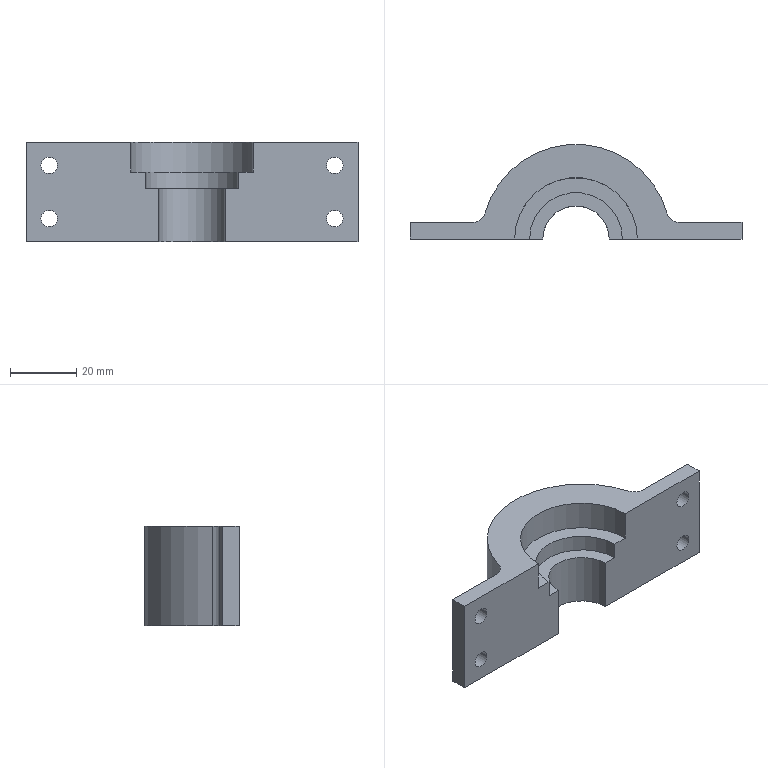Part | SolidWorks | features BaseBody 1 | 1 solid | 26 faces | box 100 x 28.5 x 30 mm | volume 35599 mm3 | cylinder 16 | plane 10 | commonest cylinder face diameters 5 x8 8 x4 20 x1 28 x1 37 x1 57 x1
STEP:
#1=CARTESIAN_POINT('',(-40.5,0.,23.));
#2=VERTEX_POINT('',#1);
#3=CARTESIAN_POINT('',(-45.5,0.,23.));
#4=VERTEX_POINT('',#3);
#5=CARTESIAN_POINT('',(-43.,0.,23.));
#6=DIRECTION('',(0.,1.,0.));
#7=DIRECTION('',(-1.,0.,0.));
#8=AXIS2_PLACEMENT_3D('',#5,#6,#7);
#9=CIRCLE('',#8,2.5);
#10=EDGE_CURVE('',#2,#4,#9,.T.);
#11=ORIENTED_EDGE('',*,*,#10,.F.);
#12=CARTESIAN_POINT('',(-40.5,5.,23.));
#13=VERTEX_POINT('',#12);
#14=CARTESIAN_POINT('',(-40.5,5.,23.));
#15=DIRECTION('',(0.,1.,0.));
#16=VECTOR('',#15,1000.);
#17=LINE('',#14,#16);
#18=EDGE_CURVE('',#2,#13,#17,.T.);
#19=ORIENTED_EDGE('',*,*,#18,.T.);
#20=CARTESIAN_POINT('',(-45.5,5.,23.));
#21=VERTEX_POINT('',#20);
#22=CARTESIAN_POINT('',(-43.,5.,23.));
#23=DIRECTION('',(0.,-1.,0.));
#24=DIRECTION('',(-1.,0.,0.));
#25=AXIS2_PLACEMENT_3D('',#22,#23,#24);
#26=CIRCLE('',#25,2.5);
#27=EDGE_CURVE('',#21,#13,#26,.T.);
#28=ORIENTED_EDGE('',*,*,#27,.F.);
#29=CARTESIAN_POINT('',(-45.5,5.,23.));
#30=DIRECTION('',(0.,1.,0.));
#31=VECTOR('',#30,1000.);
#32=LINE('',#29,#31);
#33=EDGE_CURVE('',#4,#21,#32,.T.);
#34=ORIENTED_EDGE('',*,*,#33,.F.);
#35=EDGE_LOOP('',(#11,#19,#28,#34));
#36=FACE_OUTER_BOUND('',#35,.T.);
#37=CARTESIAN_POINT('',(-43.,5.,23.));
#38=DIRECTION('',(0.,1.,0.));
#39=DIRECTION('',(-1.,0.,0.));
#40=AXIS2_PLACEMENT_3D('',#37,#38,#39);
#41=CYLINDRICAL_SURFACE('',#40,2.5);
#42=ADVANCED_FACE('',(#36),#41,.F.);
#43=CARTESIAN_POINT('',(45.5,0.,7.));
#44=VERTEX_POINT('',#43);
#45=CARTESIAN_POINT('',(40.5,0.,7.));
#46=VERTEX_POINT('',#45);
#47=CARTESIAN_POINT('',(43.,0.,7.));
#48=DIRECTION('',(0.,1.,0.));
#49=DIRECTION('',(-1.,0.,0.));
#50=AXIS2_PLACEMENT_3D('',#47,#48,#49);
#51=CIRCLE('',#50,2.5);
#52=EDGE_CURVE('',#44,#46,#51,.T.);
#53=ORIENTED_EDGE('',*,*,#52,.F.);
#54=CARTESIAN_POINT('',(45.5,5.,7.));
#55=VERTEX_POINT('',#54);
#56=CARTESIAN_POINT('',(45.5,5.,7.));
#57=DIRECTION('',(0.,1.,0.));
#58=VECTOR('',#57,1000.);
#59=LINE('',#56,#58);
#60=EDGE_CURVE('',#44,#55,#59,.T.);
#61=ORIENTED_EDGE('',*,*,#60,.T.);
#62=CARTESIAN_POINT('',(40.5,5.,7.));
#63=VERTEX_POINT('',#62);
#64=CARTESIAN_POINT('',(43.,5.,7.));
#65=DIRECTION('',(0.,-1.,0.));
#66=DIRECTION('',(-1.,0.,0.));
#67=AXIS2_PLACEMENT_3D('',#64,#65,#66);
#68=CIRCLE('',#67,2.5);
#69=EDGE_CURVE('',#63,#55,#68,.T.);
#70=ORIENTED_EDGE('',*,*,#69,.F.);
#71=CARTESIAN_POINT('',(40.5,5.,7.));
#72=DIRECTION('',(0.,1.,0.));
#73=VECTOR('',#72,1000.);
#74=LINE('',#71,#73);
#75=EDGE_CURVE('',#46,#63,#74,.T.);
#76=ORIENTED_EDGE('',*,*,#75,.F.);
#77=EDGE_LOOP('',(#53,#61,#70,#76));
#78=FACE_OUTER_BOUND('',#77,.T.);
#79=CARTESIAN_POINT('',(43.,5.,7.));
#80=DIRECTION('',(0.,1.,0.));
#81=DIRECTION('',(-1.,0.,0.));
#82=AXIS2_PLACEMENT_3D('',#79,#80,#81);
#83=CYLINDRICAL_SURFACE('',#82,2.5);
#84=ADVANCED_FACE('',(#78),#83,.F.);
#85=CARTESIAN_POINT('',(45.5,0.,23.));
#86=VERTEX_POINT('',#85);
#87=CARTESIAN_POINT('',(40.5,0.,23.));
#88=VERTEX_POINT('',#87);
#89=CARTESIAN_POINT('',(43.,0.,23.));
#90=DIRECTION('',(0.,1.,0.));
#91=DIRECTION('',(-1.,0.,0.));
#92=AXIS2_PLACEMENT_3D('',#89,#90,#91);
#93=CIRCLE('',#92,2.5);
#94=EDGE_CURVE('',#86,#88,#93,.T.);
#95=ORIENTED_EDGE('',*,*,#94,.F.);
#96=CARTESIAN_POINT('',(45.5,5.,23.));
#97=VERTEX_POINT('',#96);
#98=CARTESIAN_POINT('',(45.5,5.,23.));
#99=DIRECTION('',(0.,1.,0.));
#100=VECTOR('',#99,1000.);
#101=LINE('',#98,#100);
#102=EDGE_CURVE('',#86,#97,#101,.T.);
#103=ORIENTED_EDGE('',*,*,#102,.T.);
#104=CARTESIAN_POINT('',(40.5,5.,23.));
#105=VERTEX_POINT('',#104);
#106=CARTESIAN_POINT('',(43.,5.,23.));
#107=DIRECTION('',(0.,-1.,0.));
#108=DIRECTION('',(-1.,0.,0.));
#109=AXIS2_PLACEMENT_3D('',#106,#107,#108);
#110=CIRCLE('',#109,2.5);
#111=EDGE_CURVE('',#105,#97,#110,.T.);
#112=ORIENTED_EDGE('',*,*,#111,.F.);
#113=CARTESIAN_POINT('',(40.5,5.,23.));
#114=DIRECTION('',(0.,1.,0.));
#115=VECTOR('',#114,1000.);
#116=LINE('',#113,#115);
#117=EDGE_CURVE('',#88,#105,#116,.T.);
#118=ORIENTED_EDGE('',*,*,#117,.F.);
#119=EDGE_LOOP('',(#95,#103,#112,#118));
#120=FACE_OUTER_BOUND('',#119,.T.);
#121=CARTESIAN_POINT('',(43.,5.,23.));
#122=DIRECTION('',(0.,1.,0.));
#123=DIRECTION('',(-1.,0.,0.));
#124=AXIS2_PLACEMENT_3D('',#121,#122,#123);
#125=CYLINDRICAL_SURFACE('',#124,2.5);
#126=ADVANCED_FACE('',(#120),#125,.F.);
#127=CARTESIAN_POINT('',(-40.5,0.,7.));
#128=VERTEX_POINT('',#127);
#129=CARTESIAN_POINT('',(-45.5,0.,7.));
#130=VERTEX_POINT('',#129);
#131=CARTESIAN_POINT('',(-43.,0.,7.));
#132=DIRECTION('',(0.,1.,0.));
#133=DIRECTION('',(-1.,0.,0.));
#134=AXIS2_PLACEMENT_3D('',#131,#132,#133);
#135=CIRCLE('',#134,2.5);
#136=EDGE_CURVE('',#128,#130,#135,.T.);
#137=ORIENTED_EDGE('',*,*,#136,.F.);
#138=CARTESIAN_POINT('',(-40.5,5.,7.));
#139=VERTEX_POINT('',#138);
#140=CARTESIAN_POINT('',(-40.5,5.,7.));
#141=DIRECTION('',(0.,1.,0.));
#142=VECTOR('',#141,1000.);
#143=LINE('',#140,#142);
#144=EDGE_CURVE('',#128,#139,#143,.T.);
#145=ORIENTED_EDGE('',*,*,#144,.T.);
#146=CARTESIAN_POINT('',(-45.5,5.,7.));
#147=VERTEX_POINT('',#146);
#148=CARTESIAN_POINT('',(-43.,5.,7.));
#149=DIRECTION('',(0.,-1.,0.));
#150=DIRECTION('',(-1.,0.,0.));
#151=AXIS2_PLACEMENT_3D('',#148,#149,#150);
#152=CIRCLE('',#151,2.5);
#153=EDGE_CURVE('',#147,#139,#152,.T.);
#154=ORIENTED_EDGE('',*,*,#153,.F.);
#155=CARTESIAN_POINT('',(-45.5,5.,7.));
#156=DIRECTION('',(0.,1.,0.));
#157=VECTOR('',#156,1000.);
#158=LINE('',#155,#157);
#159=EDGE_CURVE('',#130,#147,#158,.T.);
#160=ORIENTED_EDGE('',*,*,#159,.F.);
#161=EDGE_LOOP('',(#137,#145,#154,#160));
#162=FACE_OUTER_BOUND('',#161,.T.);
#163=CARTESIAN_POINT('',(-43.,5.,7.));
#164=DIRECTION('',(0.,1.,0.));
#165=DIRECTION('',(-1.,0.,0.));
#166=AXIS2_PLACEMENT_3D('',#163,#164,#165);
#167=CYLINDRICAL_SURFACE('',#166,2.5);
#168=ADVANCED_FACE('',(#162),#167,.F.);
#169=CARTESIAN_POINT('',(-27.385,7.892,0.));
#170=VERTEX_POINT('',#169);
#171=CARTESIAN_POINT('',(-28.824,5.804,0.));
#172=VERTEX_POINT('',#171);
#173=CARTESIAN_POINT('',(-31.229,9.,0.));
#174=DIRECTION('',(0.,0.,-1.));
#175=DIRECTION('',(0.6013,-0.799,0.));
#176=AXIS2_PLACEMENT_3D('',#173,#174,#175);
#177=CIRCLE('',#176,4.);
#178=EDGE_CURVE('',#170,#172,#177,.T.);
#179=ORIENTED_EDGE('',*,*,#178,.T.);
#180=CARTESIAN_POINT('',(-28.824,5.804,30.));
#181=VERTEX_POINT('',#180);
#182=CARTESIAN_POINT('',(-28.824,5.804,0.));
#183=DIRECTION('',(0.,0.,1.));
#184=VECTOR('',#183,1000.);
#185=LINE('',#182,#184);
#186=EDGE_CURVE('',#172,#181,#185,.T.);
#187=ORIENTED_EDGE('',*,*,#186,.T.);
#188=CARTESIAN_POINT('',(-27.385,7.892,30.));
#189=VERTEX_POINT('',#188);
#190=CARTESIAN_POINT('',(-31.229,9.,30.));
#191=DIRECTION('',(0.,0.,1.));
#192=DIRECTION('',(0.6013,-0.799,0.));
#193=AXIS2_PLACEMENT_3D('',#190,#191,#192);
#194=CIRCLE('',#193,4.);
#195=EDGE_CURVE('',#181,#189,#194,.T.);
#196=ORIENTED_EDGE('',*,*,#195,.T.);
#197=CARTESIAN_POINT('',(-27.385,7.892,0.));
#198=DIRECTION('',(0.,0.,-1.));
#199=VECTOR('',#198,1000.);
#200=LINE('',#197,#199);
#201=EDGE_CURVE('',#189,#170,#200,.T.);
#202=ORIENTED_EDGE('',*,*,#201,.T.);
#203=EDGE_LOOP('',(#179,#187,#196,#202));
#204=FACE_OUTER_BOUND('',#203,.T.);
#205=CARTESIAN_POINT('',(-31.229,9.,0.));
#206=DIRECTION('',(0.,0.,1.));
#207=DIRECTION('',(0.6013,-0.799,0.));
#208=AXIS2_PLACEMENT_3D('',#205,#206,#207);
#209=CYLINDRICAL_SURFACE('',#208,4.);
#210=ADVANCED_FACE('',(#204),#209,.F.);
#211=CARTESIAN_POINT('',(27.385,7.892,30.));
#212=VERTEX_POINT('',#211);
#213=CARTESIAN_POINT('',(28.824,5.804,30.));
#214=VERTEX_POINT('',#213);
#215=CARTESIAN_POINT('',(31.229,9.,30.));
#216=DIRECTION('',(0.,0.,1.));
#217=DIRECTION('',(-0.6013,-0.799,0.));
#218=AXIS2_PLACEMENT_3D('',#215,#216,#217);
#219=CIRCLE('',#218,4.);
#220=EDGE_CURVE('',#212,#214,#219,.T.);
#221=ORIENTED_EDGE('',*,*,#220,.T.);
#222=CARTESIAN_POINT('',(28.824,5.804,0.));
#223=VERTEX_POINT('',#222);
#224=CARTESIAN_POINT('',(28.824,5.804,0.));
#225=DIRECTION('',(0.,0.,-1.));
#226=VECTOR('',#225,1000.);
#227=LINE('',#224,#226);
#228=EDGE_CURVE('',#214,#223,#227,.T.);
#229=ORIENTED_EDGE('',*,*,#228,.T.);
#230=CARTESIAN_POINT('',(27.385,7.892,0.));
#231=VERTEX_POINT('',#230);
#232=CARTESIAN_POINT('',(31.229,9.,0.));
#233=DIRECTION('',(0.,0.,-1.));
#234=DIRECTION('',(-0.6013,-0.799,0.));
#235=AXIS2_PLACEMENT_3D('',#232,#233,#234);
#236=CIRCLE('',#235,4.);
#237=EDGE_CURVE('',#223,#231,#236,.T.);
#238=ORIENTED_EDGE('',*,*,#237,.T.);
#239=CARTESIAN_POINT('',(27.385,7.892,0.));
#240=DIRECTION('',(0.,0.,1.));
#241=VECTOR('',#240,1000.);
#242=LINE('',#239,#241);
#243=EDGE_CURVE('',#231,#212,#242,.T.);
#244=ORIENTED_EDGE('',*,*,#243,.T.);
#245=EDGE_LOOP('',(#221,#229,#238,#244));
#246=FACE_OUTER_BOUND('',#245,.T.);
#247=CARTESIAN_POINT('',(31.229,9.,0.));
#248=DIRECTION('',(0.,0.,-1.));
#249=DIRECTION('',(-0.6013,-0.799,0.));
#250=AXIS2_PLACEMENT_3D('',#247,#248,#249);
#251=CYLINDRICAL_SURFACE('',#250,4.);
#252=ADVANCED_FACE('',(#246),#251,.F.);
#253=ORIENTED_EDGE('',*,*,#201,.F.);
#254=CARTESIAN_POINT('',(0.,0.,30.));
#255=DIRECTION('',(0.,0.,1.));
#256=DIRECTION('',(1.,0.,0.));
#257=AXIS2_PLACEMENT_3D('',#254,#255,#256);
#258=CIRCLE('',#257,28.5);
#259=EDGE_CURVE('',#212,#189,#258,.T.);
#260=ORIENTED_EDGE('',*,*,#259,.F.);
#261=ORIENTED_EDGE('',*,*,#243,.F.);
#262=CARTESIAN_POINT('',(0.,0.,0.));
#263=DIRECTION('',(0.,0.,1.));
#264=DIRECTION('',(1.,0.,0.));
#265=AXIS2_PLACEMENT_3D('',#262,#263,#264);
#266=CIRCLE('',#265,28.5);
#267=EDGE_CURVE('',#231,#170,#266,.T.);
#268=ORIENTED_EDGE('',*,*,#267,.T.);
#269=EDGE_LOOP('',(#253,#260,#261,#268));
#270=FACE_OUTER_BOUND('',#269,.T.);
#271=CARTESIAN_POINT('',(0.,0.,0.));
#272=DIRECTION('',(0.,0.,-1.));
#273=DIRECTION('',(1.,0.,0.));
#274=AXIS2_PLACEMENT_3D('',#271,#272,#273);
#275=CYLINDRICAL_SURFACE('',#274,28.5);
#276=ADVANCED_FACE('',(#270),#275,.T.);
#277=CARTESIAN_POINT('',(10.,0.,16.));
#278=VERTEX_POINT('',#277);
#279=CARTESIAN_POINT('',(10.,0.,0.));
#280=VERTEX_POINT('',#279);
#281=CARTESIAN_POINT('',(10.,0.,16.));
#282=DIRECTION('',(0.,0.,-1.));
#283=VECTOR('',#282,1000.);
#284=LINE('',#281,#283);
#285=EDGE_CURVE('',#278,#280,#284,.T.);
#286=ORIENTED_EDGE('',*,*,#285,.F.);
#287=CARTESIAN_POINT('',(-10.,0.,16.));
#288=VERTEX_POINT('',#287);
#289=CARTESIAN_POINT('',(0.,0.,16.));
#290=DIRECTION('',(0.,0.,-1.));
#291=DIRECTION('',(-1.,0.,0.));
#292=AXIS2_PLACEMENT_3D('',#289,#290,#291);
#293=CIRCLE('',#292,10.);
#294=EDGE_CURVE('',#288,#278,#293,.T.);
#295=ORIENTED_EDGE('',*,*,#294,.F.);
#296=CARTESIAN_POINT('',(-10.,0.,0.));
#297=VERTEX_POINT('',#296);
#298=CARTESIAN_POINT('',(-10.,0.,16.));
#299=DIRECTION('',(0.,0.,1.));
#300=VECTOR('',#299,1000.);
#301=LINE('',#298,#300);
#302=EDGE_CURVE('',#297,#288,#301,.T.);
#303=ORIENTED_EDGE('',*,*,#302,.F.);
#304=CARTESIAN_POINT('',(0.,0.,0.));
#305=DIRECTION('',(0.,0.,1.));
#306=DIRECTION('',(-1.,0.,0.));
#307=AXIS2_PLACEMENT_3D('',#304,#305,#306);
#308=CIRCLE('',#307,10.);
#309=EDGE_CURVE('',#280,#297,#308,.T.);
#310=ORIENTED_EDGE('',*,*,#309,.F.);
#311=EDGE_LOOP('',(#286,#295,#303,#310));
#312=FACE_OUTER_BOUND('',#311,.T.);
#313=CARTESIAN_POINT('',(0.,0.,16.));
#314=DIRECTION('',(0.,0.,1.));
#315=DIRECTION('',(-1.,0.,0.));
#316=AXIS2_PLACEMENT_3D('',#313,#314,#315);
#317=CYLINDRICAL_SURFACE('',#316,10.);
#318=ADVANCED_FACE('',(#312),#317,.F.);
#319=ORIENTED_EDGE('',*,*,#309,.T.);
#320=CARTESIAN_POINT('',(-50.,0.,0.));
#321=VERTEX_POINT('',#320);
#322=CARTESIAN_POINT('',(-50.,0.,0.));
#323=DIRECTION('',(1.,0.,0.));
#324=VECTOR('',#323,1000.);
#325=LINE('',#322,#324);
#326=EDGE_CURVE('',#321,#297,#325,.T.);
#327=ORIENTED_EDGE('',*,*,#326,.F.);
#328=CARTESIAN_POINT('',(-50.,5.,0.));
#329=VERTEX_POINT('',#328);
#330=CARTESIAN_POINT('',(-50.,5.,0.));
#331=DIRECTION('',(0.,-1.,0.));
#332=VECTOR('',#331,1000.);
#333=LINE('',#330,#332);
#334=EDGE_CURVE('',#329,#321,#333,.T.);
#335=ORIENTED_EDGE('',*,*,#334,.F.);
#336=CARTESIAN_POINT('',(-31.229,5.,0.));
#337=VERTEX_POINT('',#336);
#338=CARTESIAN_POINT('',(50.,5.,0.));
#339=DIRECTION('',(-1.,0.,0.));
#340=VECTOR('',#339,1000.);
#341=LINE('',#338,#340);
#342=EDGE_CURVE('',#337,#329,#341,.T.);
#343=ORIENTED_EDGE('',*,*,#342,.F.);
#344=CARTESIAN_POINT('',(-31.229,9.,0.));
#345=DIRECTION('',(0.,0.,-1.));
#346=DIRECTION('',(0.6013,-0.799,0.));
#347=AXIS2_PLACEMENT_3D('',#344,#345,#346);
#348=CIRCLE('',#347,4.);
#349=EDGE_CURVE('',#172,#337,#348,.T.);
#350=ORIENTED_EDGE('',*,*,#349,.F.);
#351=ORIENTED_EDGE('',*,*,#178,.F.);
#352=ORIENTED_EDGE('',*,*,#267,.F.);
#353=ORIENTED_EDGE('',*,*,#237,.F.);
#354=CARTESIAN_POINT('',(31.229,5.,0.));
#355=VERTEX_POINT('',#354);
#356=CARTESIAN_POINT('',(31.229,9.,0.));
#357=DIRECTION('',(0.,0.,-1.));
#358=DIRECTION('',(-0.6013,-0.799,0.));
#359=AXIS2_PLACEMENT_3D('',#356,#357,#358);
#360=CIRCLE('',#359,4.);
#361=EDGE_CURVE('',#355,#223,#360,.T.);
#362=ORIENTED_EDGE('',*,*,#361,.F.);
#363=CARTESIAN_POINT('',(50.,5.,0.));
#364=VERTEX_POINT('',#363);
#365=CARTESIAN_POINT('',(50.,5.,0.));
#366=DIRECTION('',(-1.,0.,0.));
#367=VECTOR('',#366,1000.);
#368=LINE('',#365,#367);
#369=EDGE_CURVE('',#364,#355,#368,.T.);
#370=ORIENTED_EDGE('',*,*,#369,.F.);
#371=CARTESIAN_POINT('',(50.,0.,0.));
#372=VERTEX_POINT('',#371);
#373=CARTESIAN_POINT('',(50.,0.,0.));
#374=DIRECTION('',(0.,1.,0.));
#375=VECTOR('',#374,1000.);
#376=LINE('',#373,#375);
#377=EDGE_CURVE('',#372,#364,#376,.T.);
#378=ORIENTED_EDGE('',*,*,#377,.F.);
#379=CARTESIAN_POINT('',(-50.,0.,0.));
#380=DIRECTION('',(1.,0.,0.));
#381=VECTOR('',#380,1000.);
#382=LINE('',#379,#381);
#383=EDGE_CURVE('',#280,#372,#382,.T.);
#384=ORIENTED_EDGE('',*,*,#383,.F.);
#385=EDGE_LOOP('',(#319,#327,#335,#343,#350,#351,#352,#353,#362,#370,#378,#384));
#386=FACE_OUTER_BOUND('',#385,.T.);
#387=CARTESIAN_POINT('',(0.,2.5,0.));
#388=DIRECTION('',(0.,0.,1.));
#389=DIRECTION('',(1.,0.,0.));
#390=AXIS2_PLACEMENT_3D('',#387,#388,#389);
#391=PLANE('',#390);
#392=ADVANCED_FACE('',(#386),#391,.F.);
#393=CARTESIAN_POINT('',(-43.,0.,23.));
#394=DIRECTION('',(0.,1.,0.));
#395=DIRECTION('',(-1.,0.,0.));
#396=AXIS2_PLACEMENT_3D('',#393,#394,#395);
#397=CIRCLE('',#396,2.5);
#398=EDGE_CURVE('',#4,#2,#397,.T.);
#399=ORIENTED_EDGE('',*,*,#398,.T.);
#400=ORIENTED_EDGE('',*,*,#10,.T.);
#401=EDGE_LOOP('',(#399,#400));
#402=FACE_BOUND('',#401,.T.);
#403=CARTESIAN_POINT('',(-43.,0.,7.));
#404=DIRECTION('',(0.,1.,0.));
#405=DIRECTION('',(-1.,0.,0.));
#406=AXIS2_PLACEMENT_3D('',#403,#404,#405);
#407=CIRCLE('',#406,2.5);
#408=EDGE_CURVE('',#130,#128,#407,.T.);
#409=ORIENTED_EDGE('',*,*,#408,.T.);
#410=ORIENTED_EDGE('',*,*,#136,.T.);
#411=EDGE_LOOP('',(#409,#410));
#412=FACE_BOUND('',#411,.T.);
#413=ORIENTED_EDGE('',*,*,#302,.T.);
#414=CARTESIAN_POINT('',(-14.,0.,16.));
#415=VERTEX_POINT('',#414);
#416=CARTESIAN_POINT('',(-25.,0.,16.));
#417=DIRECTION('',(-1.,0.,0.));
#418=VECTOR('',#417,1000.);
#419=LINE('',#416,#418);
#420=EDGE_CURVE('',#288,#415,#419,.T.);
#421=ORIENTED_EDGE('',*,*,#420,.T.);
#422=CARTESIAN_POINT('',(-14.,0.,21.));
#423=VERTEX_POINT('',#422);
#424=CARTESIAN_POINT('',(-14.,0.,21.));
#425=DIRECTION('',(0.,0.,1.));
#426=VECTOR('',#425,1000.);
#427=LINE('',#424,#426);
#428=EDGE_CURVE('',#415,#423,#427,.T.);
#429=ORIENTED_EDGE('',*,*,#428,.T.);
#430=CARTESIAN_POINT('',(-18.5,0.,21.));
#431=VERTEX_POINT('',#430);
#432=CARTESIAN_POINT('',(-25.,0.,21.));
#433=DIRECTION('',(-1.,0.,0.));
#434=VECTOR('',#433,1000.);
#435=LINE('',#432,#434);
#436=EDGE_CURVE('',#423,#431,#435,.T.);
#437=ORIENTED_EDGE('',*,*,#436,.T.);
#438=CARTESIAN_POINT('',(-18.5,0.,30.));
#439=VERTEX_POINT('',#438);
#440=CARTESIAN_POINT('',(-18.5,0.,30.));
#441=DIRECTION('',(0.,0.,1.));
#442=VECTOR('',#441,1000.);
#443=LINE('',#440,#442);
#444=EDGE_CURVE('',#431,#439,#443,.T.);
#445=ORIENTED_EDGE('',*,*,#444,.T.);
#446=CARTESIAN_POINT('',(-50.,0.,30.));
#447=VERTEX_POINT('',#446);
#448=CARTESIAN_POINT('',(-50.,0.,30.));
#449=DIRECTION('',(1.,0.,0.));
#450=VECTOR('',#449,1000.);
#451=LINE('',#448,#450);
#452=EDGE_CURVE('',#447,#439,#451,.T.);
#453=ORIENTED_EDGE('',*,*,#452,.F.);
#454=CARTESIAN_POINT('',(-50.,0.,0.));
#455=DIRECTION('',(0.,0.,1.));
#456=VECTOR('',#455,1000.);
#457=LINE('',#454,#456);
#458=EDGE_CURVE('',#321,#447,#457,.T.);
#459=ORIENTED_EDGE('',*,*,#458,.F.);
#460=ORIENTED_EDGE('',*,*,#326,.T.);
#461=EDGE_LOOP('',(#413,#421,#429,#437,#445,#453,#459,#460));
#462=FACE_OUTER_BOUND('',#461,.T.);
#463=CARTESIAN_POINT('',(-50.,0.,0.));
#464=DIRECTION('',(0.,-1.,0.));
#465=DIRECTION('',(-1.,0.,0.));
#466=AXIS2_PLACEMENT_3D('',#463,#464,#465);
#467=PLANE('',#466);
#468=ADVANCED_FACE('',(#402,#412,#462),#467,.T.);
#469=ORIENTED_EDGE('',*,*,#294,.T.);
#470=CARTESIAN_POINT('',(14.,0.,16.));
#471=VERTEX_POINT('',#470);
#472=CARTESIAN_POINT('',(-25.,0.,16.));
#473=DIRECTION('',(-1.,0.,0.));
#474=VECTOR('',#473,1000.);
#475=LINE('',#472,#474);
#476=EDGE_CURVE('',#471,#278,#475,.T.);
#477=ORIENTED_EDGE('',*,*,#476,.F.);
#478=CARTESIAN_POINT('',(0.,0.,16.));
#479=DIRECTION('',(0.,0.,-1.));
#480=DIRECTION('',(-1.,0.,0.));
#481=AXIS2_PLACEMENT_3D('',#478,#479,#480);
#482=CIRCLE('',#481,14.);
#483=EDGE_CURVE('',#415,#471,#482,.T.);
#484=ORIENTED_EDGE('',*,*,#483,.F.);
#485=ORIENTED_EDGE('',*,*,#420,.F.);
#486=EDGE_LOOP('',(#469,#477,#484,#485));
#487=FACE_OUTER_BOUND('',#486,.T.);
#488=CARTESIAN_POINT('',(0.,0.,16.));
#489=DIRECTION('',(0.,0.,1.));
#490=DIRECTION('',(1.,0.,0.));
#491=AXIS2_PLACEMENT_3D('',#488,#489,#490);
#492=PLANE('',#491);
#493=ADVANCED_FACE('',(#487),#492,.T.);
#494=CARTESIAN_POINT('',(14.,0.,21.));
#495=VERTEX_POINT('',#494);
#496=CARTESIAN_POINT('',(14.,0.,21.));
#497=DIRECTION('',(0.,0.,-1.));
#498=VECTOR('',#497,1000.);
#499=LINE('',#496,#498);
#500=EDGE_CURVE('',#495,#471,#499,.T.);
#501=ORIENTED_EDGE('',*,*,#500,.F.);
#502=CARTESIAN_POINT('',(0.,0.,21.));
#503=DIRECTION('',(0.,0.,-1.));
#504=DIRECTION('',(-1.,0.,0.));
#505=AXIS2_PLACEMENT_3D('',#502,#503,#504);
#506=CIRCLE('',#505,14.);
#507=EDGE_CURVE('',#423,#495,#506,.T.);
#508=ORIENTED_EDGE('',*,*,#507,.F.);
#509=ORIENTED_EDGE('',*,*,#428,.F.);
#510=ORIENTED_EDGE('',*,*,#483,.T.);
#511=EDGE_LOOP('',(#501,#508,#509,#510));
#512=FACE_OUTER_BOUND('',#511,.T.);
#513=CARTESIAN_POINT('',(0.,0.,21.));
#514=DIRECTION('',(0.,0.,1.));
#515=DIRECTION('',(-1.,0.,0.));
#516=AXIS2_PLACEMENT_3D('',#513,#514,#515);
#517=CYLINDRICAL_SURFACE('',#516,14.);
#518=ADVANCED_FACE('',(#512),#517,.F.);
#519=CARTESIAN_POINT('',(43.,0.,7.));
#520=DIRECTION('',(0.,1.,0.));
#521=DIRECTION('',(-1.,0.,0.));
#522=AXIS2_PLACEMENT_3D('',#519,#520,#521);
#523=CIRCLE('',#522,2.5);
#524=EDGE_CURVE('',#46,#44,#523,.T.);
#525=ORIENTED_EDGE('',*,*,#524,.T.);
#526=ORIENTED_EDGE('',*,*,#52,.T.);
#527=EDGE_LOOP('',(#525,#526));
#528=FACE_BOUND('',#527,.T.);
#529=CARTESIAN_POINT('',(43.,0.,23.));
#530=DIRECTION('',(0.,1.,0.));
#531=DIRECTION('',(-1.,0.,0.));
#532=AXIS2_PLACEMENT_3D('',#529,#530,#531);
#533=CIRCLE('',#532,2.5);
#534=EDGE_CURVE('',#88,#86,#533,.T.);
#535=ORIENTED_EDGE('',*,*,#534,.T.);
#536=ORIENTED_EDGE('',*,*,#94,.T.);
#537=EDGE_LOOP('',(#535,#536));
#538=FACE_BOUND('',#537,.T.);
#539=ORIENTED_EDGE('',*,*,#285,.T.);
#540=ORIENTED_EDGE('',*,*,#383,.T.);
#541=CARTESIAN_POINT('',(50.,0.,30.));
#542=VERTEX_POINT('',#541);
#543=CARTESIAN_POINT('',(50.,0.,0.));
#544=DIRECTION('',(0.,0.,1.));
#545=VECTOR('',#544,1000.);
#546=LINE('',#543,#545);
#547=EDGE_CURVE('',#372,#542,#546,.T.);
#548=ORIENTED_EDGE('',*,*,#547,.T.);
#549=CARTESIAN_POINT('',(18.5,0.,30.));
#550=VERTEX_POINT('',#549);
#551=CARTESIAN_POINT('',(-50.,0.,30.));
#552=DIRECTION('',(1.,0.,0.));
#553=VECTOR('',#552,1000.);
#554=LINE('',#551,#553);
#555=EDGE_CURVE('',#550,#542,#554,.T.);
#556=ORIENTED_EDGE('',*,*,#555,.F.);
#557=CARTESIAN_POINT('',(18.5,0.,21.));
#558=VERTEX_POINT('',#557);
#559=CARTESIAN_POINT('',(18.5,0.,30.));
#560=DIRECTION('',(0.,0.,-1.));
#561=VECTOR('',#560,1000.);
#562=LINE('',#559,#561);
#563=EDGE_CURVE('',#550,#558,#562,.T.);
#564=ORIENTED_EDGE('',*,*,#563,.T.);
#565=CARTESIAN_POINT('',(-25.,0.,21.));
#566=DIRECTION('',(-1.,0.,0.));
#567=VECTOR('',#566,1000.);
#568=LINE('',#565,#567);
#569=EDGE_CURVE('',#558,#495,#568,.T.);
#570=ORIENTED_EDGE('',*,*,#569,.T.);
#571=ORIENTED_EDGE('',*,*,#500,.T.);
#572=ORIENTED_EDGE('',*,*,#476,.T.);
#573=EDGE_LOOP('',(#539,#540,#548,#556,#564,#570,#571,#572));
#574=FACE_OUTER_BOUND('',#573,.T.);
#575=CARTESIAN_POINT('',(-50.,0.,0.));
#576=DIRECTION('',(0.,-1.,0.));
#577=DIRECTION('',(-1.,0.,0.));
#578=AXIS2_PLACEMENT_3D('',#575,#576,#577);
#579=PLANE('',#578);
#580=ADVANCED_FACE('',(#528,#538,#574),#579,.T.);
#581=ORIENTED_EDGE('',*,*,#507,.T.);
#582=ORIENTED_EDGE('',*,*,#569,.F.);
#583=CARTESIAN_POINT('',(0.,0.,21.));
#584=DIRECTION('',(0.,0.,-1.));
#585=DIRECTION('',(-1.,0.,0.));
#586=AXIS2_PLACEMENT_3D('',#583,#584,#585);
#587=CIRCLE('',#586,18.5);
#588=EDGE_CURVE('',#431,#558,#587,.T.);
#589=ORIENTED_EDGE('',*,*,#588,.F.);
#590=ORIENTED_EDGE('',*,*,#436,.F.);
#591=EDGE_LOOP('',(#581,#582,#589,#590));
#592=FACE_OUTER_BOUND('',#591,.T.);
#593=CARTESIAN_POINT('',(0.,0.,21.));
#594=DIRECTION('',(0.,0.,1.));
#595=DIRECTION('',(1.,0.,0.));
#596=AXIS2_PLACEMENT_3D('',#593,#594,#595);
#597=PLANE('',#596);
#598=ADVANCED_FACE('',(#592),#597,.T.);
#599=ORIENTED_EDGE('',*,*,#563,.F.);
#600=CARTESIAN_POINT('',(0.,0.,30.));
#601=DIRECTION('',(0.,0.,-1.));
#602=DIRECTION('',(-1.,0.,0.));
#603=AXIS2_PLACEMENT_3D('',#600,#601,#602);
#604=CIRCLE('',#603,18.5);
#605=EDGE_CURVE('',#439,#550,#604,.T.);
#606=ORIENTED_EDGE('',*,*,#605,.F.);
#607=ORIENTED_EDGE('',*,*,#444,.F.);
#608=ORIENTED_EDGE('',*,*,#588,.T.);
#609=EDGE_LOOP('',(#599,#606,#607,#608));
#610=FACE_OUTER_BOUND('',#609,.T.);
#611=CARTESIAN_POINT('',(0.,0.,30.));
#612=DIRECTION('',(0.,0.,1.));
#613=DIRECTION('',(-1.,0.,0.));
#614=AXIS2_PLACEMENT_3D('',#611,#612,#613);
#615=CYLINDRICAL_SURFACE('',#614,18.5);
#616=ADVANCED_FACE('',(#610),#615,.F.);
#617=ORIENTED_EDGE('',*,*,#605,.T.);
#618=ORIENTED_EDGE('',*,*,#555,.T.);
#619=CARTESIAN_POINT('',(50.,5.,30.));
#620=VERTEX_POINT('',#619);
#621=CARTESIAN_POINT('',(50.,0.,30.));
#622=DIRECTION('',(0.,1.,0.));
#623=VECTOR('',#622,1000.);
#624=LINE('',#621,#623);
#625=EDGE_CURVE('',#542,#620,#624,.T.);
#626=ORIENTED_EDGE('',*,*,#625,.T.);
#627=CARTESIAN_POINT('',(31.229,5.,30.));
#628=VERTEX_POINT('',#627);
#629=CARTESIAN_POINT('',(50.,5.,30.));
#630=DIRECTION('',(-1.,0.,0.));
#631=VECTOR('',#630,1000.);
#632=LINE('',#629,#631);
#633=EDGE_CURVE('',#620,#628,#632,.T.);
#634=ORIENTED_EDGE('',*,*,#633,.T.);
#635=CARTESIAN_POINT('',(31.229,9.,30.));
#636=DIRECTION('',(0.,0.,1.));
#637=DIRECTION('',(-0.6013,-0.799,0.));
#638=AXIS2_PLACEMENT_3D('',#635,#636,#637);
#639=CIRCLE('',#638,4.);
#640=EDGE_CURVE('',#214,#628,#639,.T.);
#641=ORIENTED_EDGE('',*,*,#640,.F.);
#642=ORIENTED_EDGE('',*,*,#220,.F.);
#643=ORIENTED_EDGE('',*,*,#259,.T.);
#644=ORIENTED_EDGE('',*,*,#195,.F.);
#645=CARTESIAN_POINT('',(-31.229,5.,30.));
#646=VERTEX_POINT('',#645);
#647=CARTESIAN_POINT('',(-31.229,9.,30.));
#648=DIRECTION('',(0.,0.,1.));
#649=DIRECTION('',(0.6013,-0.799,0.));
#650=AXIS2_PLACEMENT_3D('',#647,#648,#649);
#651=CIRCLE('',#650,4.);
#652=EDGE_CURVE('',#646,#181,#651,.T.);
#653=ORIENTED_EDGE('',*,*,#652,.F.);
#654=CARTESIAN_POINT('',(-50.,5.,30.));
#655=VERTEX_POINT('',#654);
#656=CARTESIAN_POINT('',(50.,5.,30.));
#657=DIRECTION('',(-1.,0.,0.));
#658=VECTOR('',#657,1000.);
#659=LINE('',#656,#658);
#660=EDGE_CURVE('',#646,#655,#659,.T.);
#661=ORIENTED_EDGE('',*,*,#660,.T.);
#662=CARTESIAN_POINT('',(-50.,5.,30.));
#663=DIRECTION('',(0.,-1.,0.));
#664=VECTOR('',#663,1000.);
#665=LINE('',#662,#664);
#666=EDGE_CURVE('',#655,#447,#665,.T.);
#667=ORIENTED_EDGE('',*,*,#666,.T.);
#668=ORIENTED_EDGE('',*,*,#452,.T.);
#669=EDGE_LOOP('',(#617,#618,#626,#634,#641,#642,#643,#644,#653,#661,#667,#668));
#670=FACE_OUTER_BOUND('',#669,.T.);
#671=CARTESIAN_POINT('',(0.,9.814,30.));
#672=DIRECTION('',(0.,0.,1.));
#673=DIRECTION('',(1.,0.,0.));
#674=AXIS2_PLACEMENT_3D('',#671,#672,#673);
#675=PLANE('',#674);
#676=ADVANCED_FACE('',(#670),#675,.T.);
#677=ORIENTED_EDGE('',*,*,#69,.T.);
#678=CARTESIAN_POINT('',(43.,5.,7.));
#679=DIRECTION('',(0.,-1.,0.));
#680=DIRECTION('',(-1.,0.,0.));
#681=AXIS2_PLACEMENT_3D('',#678,#679,#680);
#682=CIRCLE('',#681,2.5);
#683=EDGE_CURVE('',#55,#63,#682,.T.);
#684=ORIENTED_EDGE('',*,*,#683,.T.);
#685=EDGE_LOOP('',(#677,#684));
#686=FACE_BOUND('',#685,.T.);
#687=ORIENTED_EDGE('',*,*,#111,.T.);
#688=CARTESIAN_POINT('',(43.,5.,23.));
#689=DIRECTION('',(0.,-1.,0.));
#690=DIRECTION('',(-1.,0.,0.));
#691=AXIS2_PLACEMENT_3D('',#688,#689,#690);
#692=CIRCLE('',#691,2.5);
#693=EDGE_CURVE('',#97,#105,#692,.T.);
#694=ORIENTED_EDGE('',*,*,#693,.T.);
#695=EDGE_LOOP('',(#687,#694));
#696=FACE_BOUND('',#695,.T.);
#697=CARTESIAN_POINT('',(31.229,5.,0.));
#698=DIRECTION('',(0.,0.,-1.));
#699=VECTOR('',#698,1000.);
#700=LINE('',#697,#699);
#701=EDGE_CURVE('',#628,#355,#700,.T.);
#702=ORIENTED_EDGE('',*,*,#701,.F.);
#703=ORIENTED_EDGE('',*,*,#633,.F.);
#704=CARTESIAN_POINT('',(50.,5.,0.));
#705=DIRECTION('',(0.,0.,1.));
#706=VECTOR('',#705,1000.);
#707=LINE('',#704,#706);
#708=EDGE_CURVE('',#364,#620,#707,.T.);
#709=ORIENTED_EDGE('',*,*,#708,.F.);
#710=ORIENTED_EDGE('',*,*,#369,.T.);
#711=EDGE_LOOP('',(#702,#703,#709,#710));
#712=FACE_OUTER_BOUND('',#711,.T.);
#713=CARTESIAN_POINT('',(50.,5.,0.));
#714=DIRECTION('',(0.,1.,0.));
#715=DIRECTION('',(1.,0.,0.));
#716=AXIS2_PLACEMENT_3D('',#713,#714,#715);
#717=PLANE('',#716);
#718=ADVANCED_FACE('',(#686,#696,#712),#717,.T.);
#719=ORIENTED_EDGE('',*,*,#377,.T.);
#720=ORIENTED_EDGE('',*,*,#708,.T.);
#721=ORIENTED_EDGE('',*,*,#625,.F.);
#722=ORIENTED_EDGE('',*,*,#547,.F.);
#723=EDGE_LOOP('',(#719,#720,#721,#722));
#724=FACE_OUTER_BOUND('',#723,.T.);
#725=CARTESIAN_POINT('',(50.,0.,0.));
#726=DIRECTION('',(1.,0.,0.));
#727=DIRECTION('',(0.,1.,0.));
#728=AXIS2_PLACEMENT_3D('',#725,#726,#727);
#729=PLANE('',#728);
#730=ADVANCED_FACE('',(#724),#729,.T.);
#731=ORIENTED_EDGE('',*,*,#334,.T.);
#732=ORIENTED_EDGE('',*,*,#458,.T.);
#733=ORIENTED_EDGE('',*,*,#666,.F.);
#734=CARTESIAN_POINT('',(-50.,5.,0.));
#735=DIRECTION('',(0.,0.,1.));
#736=VECTOR('',#735,1000.);
#737=LINE('',#734,#736);
#738=EDGE_CURVE('',#329,#655,#737,.T.);
#739=ORIENTED_EDGE('',*,*,#738,.F.);
#740=EDGE_LOOP('',(#731,#732,#733,#739));
#741=FACE_OUTER_BOUND('',#740,.T.);
#742=CARTESIAN_POINT('',(-50.,5.,0.));
#743=DIRECTION('',(-1.,0.,0.));
#744=DIRECTION('',(0.,0.,1.));
#745=AXIS2_PLACEMENT_3D('',#742,#743,#744);
#746=PLANE('',#745);
#747=ADVANCED_FACE('',(#741),#746,.T.);
#748=ORIENTED_EDGE('',*,*,#27,.T.);
#749=CARTESIAN_POINT('',(-43.,5.,23.));
#750=DIRECTION('',(0.,-1.,0.));
#751=DIRECTION('',(-1.,0.,0.));
#752=AXIS2_PLACEMENT_3D('',#749,#750,#751);
#753=CIRCLE('',#752,2.5);
#754=EDGE_CURVE('',#13,#21,#753,.T.);
#755=ORIENTED_EDGE('',*,*,#754,.T.);
#756=EDGE_LOOP('',(#748,#755));
#757=FACE_BOUND('',#756,.T.);
#758=ORIENTED_EDGE('',*,*,#153,.T.);
#759=CARTESIAN_POINT('',(-43.,5.,7.));
#760=DIRECTION('',(0.,-1.,0.));
#761=DIRECTION('',(-1.,0.,0.));
#762=AXIS2_PLACEMENT_3D('',#759,#760,#761);
#763=CIRCLE('',#762,2.5);
#764=EDGE_CURVE('',#139,#147,#763,.T.);
#765=ORIENTED_EDGE('',*,*,#764,.T.);
#766=EDGE_LOOP('',(#758,#765));
#767=FACE_BOUND('',#766,.T.);
#768=CARTESIAN_POINT('',(-31.229,5.,0.));
#769=DIRECTION('',(0.,0.,1.));
#770=VECTOR('',#769,1000.);
#771=LINE('',#768,#770);
#772=EDGE_CURVE('',#337,#646,#771,.T.);
#773=ORIENTED_EDGE('',*,*,#772,.F.);
#774=ORIENTED_EDGE('',*,*,#342,.T.);
#775=ORIENTED_EDGE('',*,*,#738,.T.);
#776=ORIENTED_EDGE('',*,*,#660,.F.);
#777=EDGE_LOOP('',(#773,#774,#775,#776));
#778=FACE_OUTER_BOUND('',#777,.T.);
#779=CARTESIAN_POINT('',(50.,5.,0.));
#780=DIRECTION('',(0.,1.,0.));
#781=DIRECTION('',(1.,0.,0.));
#782=AXIS2_PLACEMENT_3D('',#779,#780,#781);
#783=PLANE('',#782);
#784=ADVANCED_FACE('',(#757,#767,#778),#783,.T.);
#785=ORIENTED_EDGE('',*,*,#228,.F.);
#786=ORIENTED_EDGE('',*,*,#640,.T.);
#787=ORIENTED_EDGE('',*,*,#701,.T.);
#788=ORIENTED_EDGE('',*,*,#361,.T.);
#789=EDGE_LOOP('',(#785,#786,#787,#788));
#790=FACE_OUTER_BOUND('',#789,.T.);
#791=CARTESIAN_POINT('',(31.229,9.,0.));
#792=DIRECTION('',(0.,0.,-1.));
#793=DIRECTION('',(-0.6013,-0.799,0.));
#794=AXIS2_PLACEMENT_3D('',#791,#792,#793);
#795=CYLINDRICAL_SURFACE('',#794,4.);
#796=ADVANCED_FACE('',(#790),#795,.F.);
#797=ORIENTED_EDGE('',*,*,#186,.F.);
#798=ORIENTED_EDGE('',*,*,#349,.T.);
#799=ORIENTED_EDGE('',*,*,#772,.T.);
#800=ORIENTED_EDGE('',*,*,#652,.T.);
#801=EDGE_LOOP('',(#797,#798,#799,#800));
#802=FACE_OUTER_BOUND('',#801,.T.);
#803=CARTESIAN_POINT('',(-31.229,9.,0.));
#804=DIRECTION('',(0.,0.,1.));
#805=DIRECTION('',(0.6013,-0.799,0.));
#806=AXIS2_PLACEMENT_3D('',#803,#804,#805);
#807=CYLINDRICAL_SURFACE('',#806,4.);
#808=ADVANCED_FACE('',(#802),#807,.F.);
#809=ORIENTED_EDGE('',*,*,#144,.F.);
#810=ORIENTED_EDGE('',*,*,#408,.F.);
#811=ORIENTED_EDGE('',*,*,#159,.T.);
#812=ORIENTED_EDGE('',*,*,#764,.F.);
#813=EDGE_LOOP('',(#809,#810,#811,#812));
#814=FACE_OUTER_BOUND('',#813,.T.);
#815=CARTESIAN_POINT('',(-43.,5.,7.));
#816=DIRECTION('',(0.,1.,0.));
#817=DIRECTION('',(-1.,0.,0.));
#818=AXIS2_PLACEMENT_3D('',#815,#816,#817);
#819=CYLINDRICAL_SURFACE('',#818,2.5);
#820=ADVANCED_FACE('',(#814),#819,.F.);
#821=ORIENTED_EDGE('',*,*,#102,.F.);
#822=ORIENTED_EDGE('',*,*,#534,.F.);
#823=ORIENTED_EDGE('',*,*,#117,.T.);
#824=ORIENTED_EDGE('',*,*,#693,.F.);
#825=EDGE_LOOP('',(#821,#822,#823,#824));
#826=FACE_OUTER_BOUND('',#825,.T.);
#827=CARTESIAN_POINT('',(43.,5.,23.));
#828=DIRECTION('',(0.,1.,0.));
#829=DIRECTION('',(-1.,0.,0.));
#830=AXIS2_PLACEMENT_3D('',#827,#828,#829);
#831=CYLINDRICAL_SURFACE('',#830,2.5);
#832=ADVANCED_FACE('',(#826),#831,.F.);
#833=ORIENTED_EDGE('',*,*,#60,.F.);
#834=ORIENTED_EDGE('',*,*,#524,.F.);
#835=ORIENTED_EDGE('',*,*,#75,.T.);
#836=ORIENTED_EDGE('',*,*,#683,.F.);
#837=EDGE_LOOP('',(#833,#834,#835,#836));
#838=FACE_OUTER_BOUND('',#837,.T.);
#839=CARTESIAN_POINT('',(43.,5.,7.));
#840=DIRECTION('',(0.,1.,0.));
#841=DIRECTION('',(-1.,0.,0.));
#842=AXIS2_PLACEMENT_3D('',#839,#840,#841);
#843=CYLINDRICAL_SURFACE('',#842,2.5);
#844=ADVANCED_FACE('',(#838),#843,.F.);
#845=ORIENTED_EDGE('',*,*,#18,.F.);
#846=ORIENTED_EDGE('',*,*,#398,.F.);
#847=ORIENTED_EDGE('',*,*,#33,.T.);
#848=ORIENTED_EDGE('',*,*,#754,.F.);
#849=EDGE_LOOP('',(#845,#846,#847,#848));
#850=FACE_OUTER_BOUND('',#849,.T.);
#851=CARTESIAN_POINT('',(-43.,5.,23.));
#852=DIRECTION('',(0.,1.,0.));
#853=DIRECTION('',(-1.,0.,0.));
#854=AXIS2_PLACEMENT_3D('',#851,#852,#853);
#855=CYLINDRICAL_SURFACE('',#854,2.5);
#856=ADVANCED_FACE('',(#850),#855,.F.);
#857=CLOSED_SHELL('',(#42,#84,#126,#168,#210,#252,#276,#318,#392,#468,#493,#518,#580,#598,#616,#676,#718,#730,#747,#784,#796,#808,#820,#832,#844,#856));
#858=MANIFOLD_SOLID_BREP('',#857);
#859=CARTESIAN_POINT('',(0.,0.,0.));
#860=DIRECTION('',(0.,0.,1.));
#861=DIRECTION('',(1.,0.,0.));
#862=AXIS2_PLACEMENT_3D('',#859,#860,#861);
#863=(LENGTH_UNIT()NAMED_UNIT(*)SI_UNIT(.MILLI.,.METRE.));
#864=UNCERTAINTY_MEASURE_WITH_UNIT(LENGTH_MEASURE(0.00001),#863,'','');
#865=(NAMED_UNIT(*)PLANE_ANGLE_UNIT()SI_UNIT($,.RADIAN.));
#866=(NAMED_UNIT(*)SI_UNIT($,.STERADIAN.)SOLID_ANGLE_UNIT());
#867=(GEOMETRIC_REPRESENTATION_CONTEXT(3)GLOBAL_UNCERTAINTY_ASSIGNED_CONTEXT((#864))GLOBAL_UNIT_ASSIGNED_CONTEXT((#863,#865,#866))REPRESENTATION_CONTEXT('',''));
#868=ADVANCED_BREP_SHAPE_REPRESENTATION('',(#858,#862),#867);